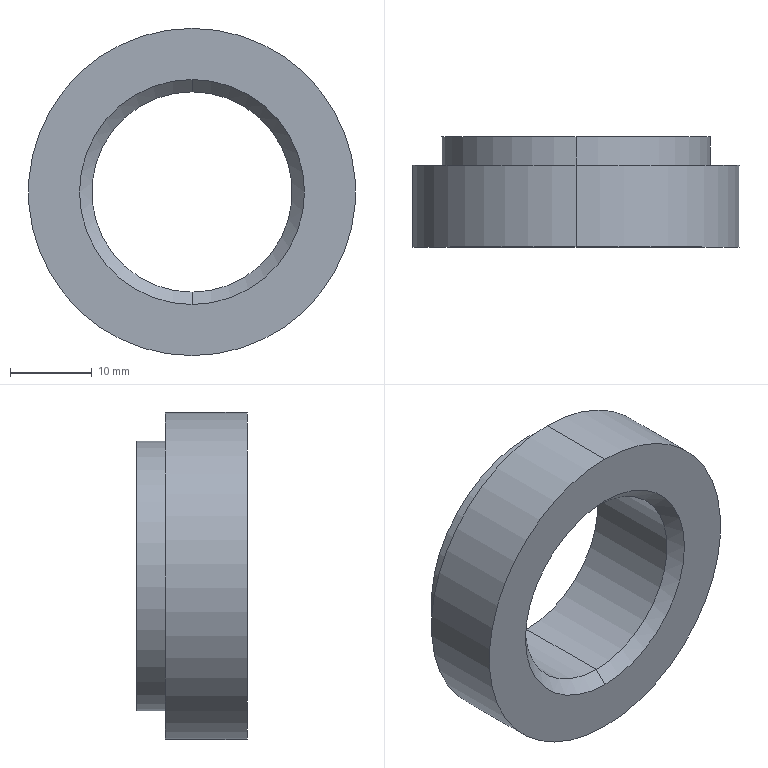Part | SolidWorks | features Chamfer 1, HoleWzd 1, Revolution 1 | 1 solid | 11 faces | box 40 x 13.5 x 40 mm | volume 9105 mm3 | cylinder 6 | plane 3 | cone 2 | commonest cylinder face diameters 24.5 x2 33 x2 40 x2
STEP:
#1=CARTESIAN_POINT('',(0.,1.5,12.25));
#2=VERTEX_POINT('',#1);
#3=CARTESIAN_POINT('',(0.,1.5,-12.25));
#4=VERTEX_POINT('',#3);
#5=CARTESIAN_POINT('',(0.,1.5,0.));
#6=DIRECTION('',(0.,-1.,0.));
#7=DIRECTION('',(0.,0.,-1.));
#8=AXIS2_PLACEMENT_3D('',#5,#6,#7);
#9=CIRCLE('',#8,12.25);
#10=EDGE_CURVE('',#2,#4,#9,.T.);
#11=ORIENTED_EDGE('',*,*,#10,.F.);
#12=CARTESIAN_POINT('',(0.,0.,13.75));
#13=VERTEX_POINT('',#12);
#14=CARTESIAN_POINT('',(0.,1.5,12.25));
#15=DIRECTION('',(0.,-0.7071,0.7071));
#16=VECTOR('',#15,1000.);
#17=LINE('',#14,#16);
#18=EDGE_CURVE('',#2,#13,#17,.T.);
#19=ORIENTED_EDGE('',*,*,#18,.T.);
#20=CARTESIAN_POINT('',(0.,0.,-13.75));
#21=VERTEX_POINT('',#20);
#22=CARTESIAN_POINT('',(0.,0.,0.));
#23=DIRECTION('',(0.,1.,0.));
#24=DIRECTION('',(0.,0.,-1.));
#25=AXIS2_PLACEMENT_3D('',#22,#23,#24);
#26=CIRCLE('',#25,13.75);
#27=EDGE_CURVE('',#21,#13,#26,.T.);
#28=ORIENTED_EDGE('',*,*,#27,.F.);
#29=CARTESIAN_POINT('',(0.,1.5,-12.25));
#30=DIRECTION('',(0.,-0.7071,-0.7071));
#31=VECTOR('',#30,1000.);
#32=LINE('',#29,#31);
#33=EDGE_CURVE('',#4,#21,#32,.T.);
#34=ORIENTED_EDGE('',*,*,#33,.F.);
#35=EDGE_LOOP('',(#11,#19,#28,#34));
#36=FACE_OUTER_BOUND('',#35,.T.);
#37=CARTESIAN_POINT('',(0.,1.5,0.));
#38=DIRECTION('',(0.,-1.,0.));
#39=DIRECTION('',(0.,0.,-1.));
#40=AXIS2_PLACEMENT_3D('',#37,#38,#39);
#41=CONICAL_SURFACE('',#40,12.25,0.7854);
#42=ADVANCED_FACE('',(#36),#41,.F.);
#43=ORIENTED_EDGE('',*,*,#10,.T.);
#44=CARTESIAN_POINT('',(0.,13.5,-12.25));
#45=VERTEX_POINT('',#44);
#46=CARTESIAN_POINT('',(0.,13.5,-12.25));
#47=DIRECTION('',(0.,1.,0.));
#48=VECTOR('',#47,1000.);
#49=LINE('',#46,#48);
#50=EDGE_CURVE('',#4,#45,#49,.T.);
#51=ORIENTED_EDGE('',*,*,#50,.T.);
#52=CARTESIAN_POINT('',(0.,13.5,12.25));
#53=VERTEX_POINT('',#52);
#54=CARTESIAN_POINT('',(0.,13.5,0.));
#55=DIRECTION('',(0.,1.,0.));
#56=DIRECTION('',(0.,0.,1.));
#57=AXIS2_PLACEMENT_3D('',#54,#55,#56);
#58=CIRCLE('',#57,12.25);
#59=EDGE_CURVE('',#45,#53,#58,.T.);
#60=ORIENTED_EDGE('',*,*,#59,.T.);
#61=CARTESIAN_POINT('',(0.,13.5,12.25));
#62=DIRECTION('',(0.,1.,0.));
#63=VECTOR('',#62,1000.);
#64=LINE('',#61,#63);
#65=EDGE_CURVE('',#2,#53,#64,.T.);
#66=ORIENTED_EDGE('',*,*,#65,.F.);
#67=EDGE_LOOP('',(#43,#51,#60,#66));
#68=FACE_OUTER_BOUND('',#67,.T.);
#69=CARTESIAN_POINT('',(0.,13.5,0.));
#70=DIRECTION('',(0.,1.,0.));
#71=DIRECTION('',(0.,0.,1.));
#72=AXIS2_PLACEMENT_3D('',#69,#70,#71);
#73=CYLINDRICAL_SURFACE('',#72,12.25);
#74=ADVANCED_FACE('',(#68),#73,.F.);
#75=CARTESIAN_POINT('',(0.,13.5,-16.5));
#76=VERTEX_POINT('',#75);
#77=CARTESIAN_POINT('',(0.,13.5,16.5));
#78=VERTEX_POINT('',#77);
#79=CARTESIAN_POINT('',(0.,13.5,0.));
#80=DIRECTION('',(0.,-1.,0.));
#81=DIRECTION('',(0.,0.,-1.));
#82=AXIS2_PLACEMENT_3D('',#79,#80,#81);
#83=CIRCLE('',#82,16.5);
#84=EDGE_CURVE('',#76,#78,#83,.T.);
#85=ORIENTED_EDGE('',*,*,#84,.T.);
#86=CARTESIAN_POINT('',(0.,10.,16.5));
#87=VERTEX_POINT('',#86);
#88=CARTESIAN_POINT('',(0.,0.,16.5));
#89=DIRECTION('',(0.,-1.,0.));
#90=VECTOR('',#89,1000.);
#91=LINE('',#88,#90);
#92=EDGE_CURVE('',#78,#87,#91,.T.);
#93=ORIENTED_EDGE('',*,*,#92,.T.);
#94=CARTESIAN_POINT('',(0.,10.,-16.5));
#95=VERTEX_POINT('',#94);
#96=CARTESIAN_POINT('',(0.,10.,0.));
#97=DIRECTION('',(0.,-1.,0.));
#98=DIRECTION('',(0.,0.,-1.));
#99=AXIS2_PLACEMENT_3D('',#96,#97,#98);
#100=CIRCLE('',#99,16.5);
#101=EDGE_CURVE('',#95,#87,#100,.T.);
#102=ORIENTED_EDGE('',*,*,#101,.F.);
#103=CARTESIAN_POINT('',(0.,0.,-16.5));
#104=DIRECTION('',(0.,-1.,0.));
#105=VECTOR('',#104,1000.);
#106=LINE('',#103,#105);
#107=EDGE_CURVE('',#76,#95,#106,.T.);
#108=ORIENTED_EDGE('',*,*,#107,.F.);
#109=EDGE_LOOP('',(#85,#93,#102,#108));
#110=FACE_OUTER_BOUND('',#109,.T.);
#111=CARTESIAN_POINT('',(0.,0.,0.));
#112=DIRECTION('',(0.,-1.,0.));
#113=DIRECTION('',(0.,0.,-1.));
#114=AXIS2_PLACEMENT_3D('',#111,#112,#113);
#115=CYLINDRICAL_SURFACE('',#114,16.5);
#116=ADVANCED_FACE('',(#110),#115,.T.);
#117=CARTESIAN_POINT('',(0.,10.,-20.));
#118=VERTEX_POINT('',#117);
#119=CARTESIAN_POINT('',(0.,10.,20.));
#120=VERTEX_POINT('',#119);
#121=CARTESIAN_POINT('',(0.,10.,0.));
#122=DIRECTION('',(0.,-1.,0.));
#123=DIRECTION('',(0.,0.,-1.));
#124=AXIS2_PLACEMENT_3D('',#121,#122,#123);
#125=CIRCLE('',#124,20.);
#126=EDGE_CURVE('',#118,#120,#125,.T.);
#127=ORIENTED_EDGE('',*,*,#126,.T.);
#128=CARTESIAN_POINT('',(0.,0.,20.));
#129=VERTEX_POINT('',#128);
#130=CARTESIAN_POINT('',(0.,0.,20.));
#131=DIRECTION('',(0.,-1.,0.));
#132=VECTOR('',#131,1000.);
#133=LINE('',#130,#132);
#134=EDGE_CURVE('',#120,#129,#133,.T.);
#135=ORIENTED_EDGE('',*,*,#134,.T.);
#136=CARTESIAN_POINT('',(0.,0.,-20.));
#137=VERTEX_POINT('',#136);
#138=CARTESIAN_POINT('',(0.,0.,0.));
#139=DIRECTION('',(0.,-1.,0.));
#140=DIRECTION('',(0.,0.,-1.));
#141=AXIS2_PLACEMENT_3D('',#138,#139,#140);
#142=CIRCLE('',#141,20.);
#143=EDGE_CURVE('',#137,#129,#142,.T.);
#144=ORIENTED_EDGE('',*,*,#143,.F.);
#145=CARTESIAN_POINT('',(0.,0.,-20.));
#146=DIRECTION('',(0.,-1.,0.));
#147=VECTOR('',#146,1000.);
#148=LINE('',#145,#147);
#149=EDGE_CURVE('',#118,#137,#148,.T.);
#150=ORIENTED_EDGE('',*,*,#149,.F.);
#151=EDGE_LOOP('',(#127,#135,#144,#150));
#152=FACE_OUTER_BOUND('',#151,.T.);
#153=CARTESIAN_POINT('',(0.,0.,0.));
#154=DIRECTION('',(0.,-1.,0.));
#155=DIRECTION('',(0.,0.,-1.));
#156=AXIS2_PLACEMENT_3D('',#153,#154,#155);
#157=CYLINDRICAL_SURFACE('',#156,20.);
#158=ADVANCED_FACE('',(#152),#157,.T.);
#159=ORIENTED_EDGE('',*,*,#27,.T.);
#160=CARTESIAN_POINT('',(0.,0.,0.));
#161=DIRECTION('',(0.,1.,0.));
#162=DIRECTION('',(0.,0.,-1.));
#163=AXIS2_PLACEMENT_3D('',#160,#161,#162);
#164=CIRCLE('',#163,13.75);
#165=EDGE_CURVE('',#13,#21,#164,.T.);
#166=ORIENTED_EDGE('',*,*,#165,.T.);
#167=EDGE_LOOP('',(#159,#166));
#168=FACE_BOUND('',#167,.T.);
#169=ORIENTED_EDGE('',*,*,#143,.T.);
#170=CARTESIAN_POINT('',(0.,0.,0.));
#171=DIRECTION('',(0.,-1.,0.));
#172=DIRECTION('',(0.,0.,-1.));
#173=AXIS2_PLACEMENT_3D('',#170,#171,#172);
#174=CIRCLE('',#173,20.);
#175=EDGE_CURVE('',#129,#137,#174,.T.);
#176=ORIENTED_EDGE('',*,*,#175,.T.);
#177=EDGE_LOOP('',(#169,#176));
#178=FACE_OUTER_BOUND('',#177,.T.);
#179=CARTESIAN_POINT('',(0.,0.,0.));
#180=DIRECTION('',(0.,-1.,0.));
#181=DIRECTION('',(0.,0.,-1.));
#182=AXIS2_PLACEMENT_3D('',#179,#180,#181);
#183=PLANE('',#182);
#184=ADVANCED_FACE('',(#168,#178),#183,.T.);
#185=ORIENTED_EDGE('',*,*,#134,.F.);
#186=CARTESIAN_POINT('',(0.,10.,0.));
#187=DIRECTION('',(0.,-1.,0.));
#188=DIRECTION('',(0.,0.,-1.));
#189=AXIS2_PLACEMENT_3D('',#186,#187,#188);
#190=CIRCLE('',#189,20.);
#191=EDGE_CURVE('',#120,#118,#190,.T.);
#192=ORIENTED_EDGE('',*,*,#191,.T.);
#193=ORIENTED_EDGE('',*,*,#149,.T.);
#194=ORIENTED_EDGE('',*,*,#175,.F.);
#195=EDGE_LOOP('',(#185,#192,#193,#194));
#196=FACE_OUTER_BOUND('',#195,.T.);
#197=CARTESIAN_POINT('',(0.,0.,0.));
#198=DIRECTION('',(0.,-1.,0.));
#199=DIRECTION('',(0.,0.,-1.));
#200=AXIS2_PLACEMENT_3D('',#197,#198,#199);
#201=CYLINDRICAL_SURFACE('',#200,20.);
#202=ADVANCED_FACE('',(#196),#201,.T.);
#203=ORIENTED_EDGE('',*,*,#101,.T.);
#204=CARTESIAN_POINT('',(0.,10.,0.));
#205=DIRECTION('',(0.,-1.,0.));
#206=DIRECTION('',(0.,0.,-1.));
#207=AXIS2_PLACEMENT_3D('',#204,#205,#206);
#208=CIRCLE('',#207,16.5);
#209=EDGE_CURVE('',#87,#95,#208,.T.);
#210=ORIENTED_EDGE('',*,*,#209,.T.);
#211=EDGE_LOOP('',(#203,#210));
#212=FACE_BOUND('',#211,.T.);
#213=ORIENTED_EDGE('',*,*,#126,.F.);
#214=ORIENTED_EDGE('',*,*,#191,.F.);
#215=EDGE_LOOP('',(#213,#214));
#216=FACE_OUTER_BOUND('',#215,.T.);
#217=CARTESIAN_POINT('',(20.,10.,0.));
#218=DIRECTION('',(0.,1.,0.));
#219=DIRECTION('',(0.,0.,1.));
#220=AXIS2_PLACEMENT_3D('',#217,#218,#219);
#221=PLANE('',#220);
#222=ADVANCED_FACE('',(#212,#216),#221,.T.);
#223=ORIENTED_EDGE('',*,*,#92,.F.);
#224=CARTESIAN_POINT('',(0.,13.5,0.));
#225=DIRECTION('',(0.,-1.,0.));
#226=DIRECTION('',(0.,0.,-1.));
#227=AXIS2_PLACEMENT_3D('',#224,#225,#226);
#228=CIRCLE('',#227,16.5);
#229=EDGE_CURVE('',#78,#76,#228,.T.);
#230=ORIENTED_EDGE('',*,*,#229,.T.);
#231=ORIENTED_EDGE('',*,*,#107,.T.);
#232=ORIENTED_EDGE('',*,*,#209,.F.);
#233=EDGE_LOOP('',(#223,#230,#231,#232));
#234=FACE_OUTER_BOUND('',#233,.T.);
#235=CARTESIAN_POINT('',(0.,0.,0.));
#236=DIRECTION('',(0.,-1.,0.));
#237=DIRECTION('',(0.,0.,-1.));
#238=AXIS2_PLACEMENT_3D('',#235,#236,#237);
#239=CYLINDRICAL_SURFACE('',#238,16.5);
#240=ADVANCED_FACE('',(#234),#239,.T.);
#241=CARTESIAN_POINT('',(0.,13.5,0.));
#242=DIRECTION('',(0.,1.,0.));
#243=DIRECTION('',(0.,0.,1.));
#244=AXIS2_PLACEMENT_3D('',#241,#242,#243);
#245=CIRCLE('',#244,12.25);
#246=EDGE_CURVE('',#53,#45,#245,.T.);
#247=ORIENTED_EDGE('',*,*,#246,.F.);
#248=ORIENTED_EDGE('',*,*,#59,.F.);
#249=EDGE_LOOP('',(#247,#248));
#250=FACE_BOUND('',#249,.T.);
#251=ORIENTED_EDGE('',*,*,#84,.F.);
#252=ORIENTED_EDGE('',*,*,#229,.F.);
#253=EDGE_LOOP('',(#251,#252));
#254=FACE_OUTER_BOUND('',#253,.T.);
#255=CARTESIAN_POINT('',(16.5,13.5,0.));
#256=DIRECTION('',(0.,1.,0.));
#257=DIRECTION('',(0.,0.,1.));
#258=AXIS2_PLACEMENT_3D('',#255,#256,#257);
#259=PLANE('',#258);
#260=ADVANCED_FACE('',(#250,#254),#259,.T.);
#261=ORIENTED_EDGE('',*,*,#50,.F.);
#262=CARTESIAN_POINT('',(0.,1.5,0.));
#263=DIRECTION('',(0.,-1.,0.));
#264=DIRECTION('',(0.,0.,-1.));
#265=AXIS2_PLACEMENT_3D('',#262,#263,#264);
#266=CIRCLE('',#265,12.25);
#267=EDGE_CURVE('',#4,#2,#266,.T.);
#268=ORIENTED_EDGE('',*,*,#267,.T.);
#269=ORIENTED_EDGE('',*,*,#65,.T.);
#270=ORIENTED_EDGE('',*,*,#246,.T.);
#271=EDGE_LOOP('',(#261,#268,#269,#270));
#272=FACE_OUTER_BOUND('',#271,.T.);
#273=CARTESIAN_POINT('',(0.,13.5,0.));
#274=DIRECTION('',(0.,1.,0.));
#275=DIRECTION('',(0.,0.,1.));
#276=AXIS2_PLACEMENT_3D('',#273,#274,#275);
#277=CYLINDRICAL_SURFACE('',#276,12.25);
#278=ADVANCED_FACE('',(#272),#277,.F.);
#279=ORIENTED_EDGE('',*,*,#18,.F.);
#280=ORIENTED_EDGE('',*,*,#267,.F.);
#281=ORIENTED_EDGE('',*,*,#33,.T.);
#282=ORIENTED_EDGE('',*,*,#165,.F.);
#283=EDGE_LOOP('',(#279,#280,#281,#282));
#284=FACE_OUTER_BOUND('',#283,.T.);
#285=CARTESIAN_POINT('',(0.,1.5,0.));
#286=DIRECTION('',(0.,-1.,0.));
#287=DIRECTION('',(0.,0.,-1.));
#288=AXIS2_PLACEMENT_3D('',#285,#286,#287);
#289=CONICAL_SURFACE('',#288,12.25,0.7854);
#290=ADVANCED_FACE('',(#284),#289,.F.);
#291=CLOSED_SHELL('',(#42,#74,#116,#158,#184,#202,#222,#240,#260,#278,#290));
#292=MANIFOLD_SOLID_BREP('',#291);
#293=CARTESIAN_POINT('',(0.,0.,0.));
#294=DIRECTION('',(0.,0.,1.));
#295=DIRECTION('',(1.,0.,0.));
#296=AXIS2_PLACEMENT_3D('',#293,#294,#295);
#297=(LENGTH_UNIT()NAMED_UNIT(*)SI_UNIT(.MILLI.,.METRE.));
#298=UNCERTAINTY_MEASURE_WITH_UNIT(LENGTH_MEASURE(0.00001),#297,'','');
#299=(NAMED_UNIT(*)PLANE_ANGLE_UNIT()SI_UNIT($,.RADIAN.));
#300=(NAMED_UNIT(*)SI_UNIT($,.STERADIAN.)SOLID_ANGLE_UNIT());
#301=(GEOMETRIC_REPRESENTATION_CONTEXT(3)GLOBAL_UNCERTAINTY_ASSIGNED_CONTEXT((#298))GLOBAL_UNIT_ASSIGNED_CONTEXT((#297,#299,#300))REPRESENTATION_CONTEXT('',''));
#302=ADVANCED_BREP_SHAPE_REPRESENTATION('',(#292,#296),#301);